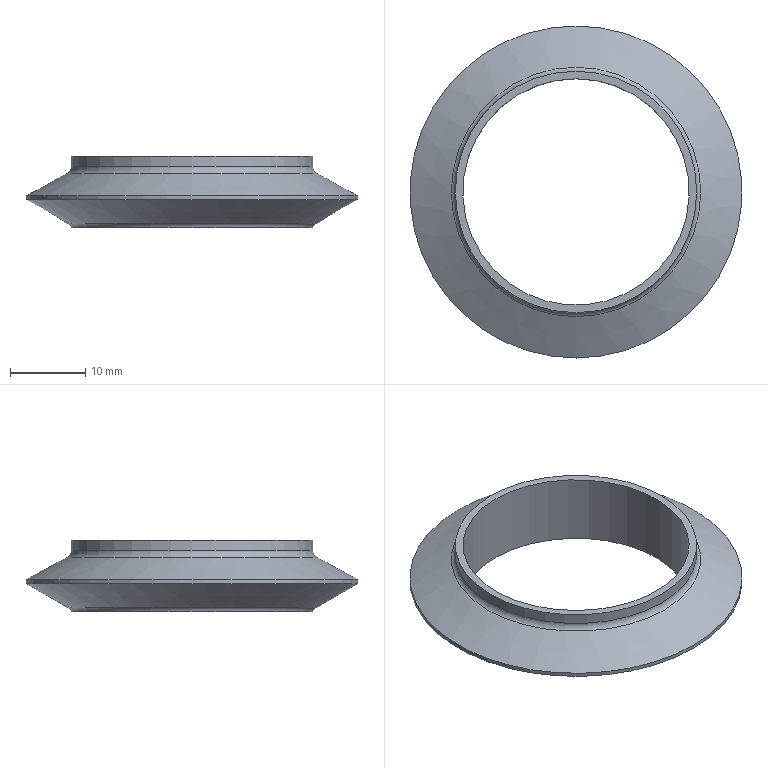Part | STEP file | 1-14.3 | 1 solid | 9 faces | box 44 x 44 x 9.5 mm | volume 3548 mm3 | cylinder 3 | cone 2 | torus 2 | plane 2 | commonest cylinder face diameters 30 x1 32 x1 44 x1
STEP:
#1=CARTESIAN_POINT('',(0.,0.,0.));
#2=DIRECTION('',(0.,0.,1.));
#3=DIRECTION('',(1.,0.,0.));
#4=AXIS2_PLACEMENT_3D('',#1,#2,#3);
#5=CARTESIAN_POINT('',(0.,22.,4.25));
#6=VERTEX_POINT('',#5);
#7=CARTESIAN_POINT('',(0.,0.,4.25));
#8=DIRECTION('',(0.,0.,1.));
#9=DIRECTION('',(0.,1.,0.));
#10=AXIS2_PLACEMENT_3D('',#7,#8,#9);
#11=CIRCLE('',#10,22.);
#12=CARTESIAN_POINT('',(0.,0.,7.216));
#13=DIRECTION('',(0.,0.,-1.));
#14=DIRECTION('',(0.,1.,0.));
#15=AXIS2_PLACEMENT_3D('',#12,#13,#14);
#16=CONICAL_SURFACE('',#15,16.524,1.074);
#17=CARTESIAN_POINT('',(6.283,2.966));
#18=DIRECTION('',(-1.,0.));
#19=VECTOR('',#18,1.);
#20=LINE('',#17,#19);
#21=(GEOMETRIC_REPRESENTATION_CONTEXT(2)PARAMETRIC_REPRESENTATION_CONTEXT()REPRESENTATION_CONTEXT('',''));
#22=DEFINITIONAL_REPRESENTATION('',(#20),#21);
#23=PCURVE('',#16,#22);
#24=CARTESIAN_POINT('',(0.,0.,3.75));
#25=DIRECTION('',(0.,0.,1.));
#26=DIRECTION('',(0.,1.,0.));
#27=AXIS2_PLACEMENT_3D('',#24,#25,#26);
#28=CYLINDRICAL_SURFACE('',#27,22.);
#29=CARTESIAN_POINT('',(0.,0.5));
#30=DIRECTION('',(1.,0.));
#31=VECTOR('',#30,1.);
#32=LINE('',#29,#31);
#33=(GEOMETRIC_REPRESENTATION_CONTEXT(2)PARAMETRIC_REPRESENTATION_CONTEXT()REPRESENTATION_CONTEXT('',''));
#34=DEFINITIONAL_REPRESENTATION('',(#32),#33);
#35=PCURVE('',#28,#34);
#36=SURFACE_CURVE('',#11,(#23,#35),.PCURVE_S1.);
#37=EDGE_CURVE('',#6,#6,#36,.T.);
#38=ORIENTED_EDGE('',*,*,#37,.T.);
#39=CARTESIAN_POINT('',(0.,16.524,7.216));
#40=VERTEX_POINT('',#39);
#41=CARTESIAN_POINT('',(0.,22.,4.25));
#42=DIRECTION('',(0.,-0.8793,0.4763));
#43=VECTOR('',#42,1.);
#44=LINE('',#41,#43);
#45=CARTESIAN_POINT('',(0.,2.966));
#46=DIRECTION('',(0.,-1.));
#47=VECTOR('',#46,1.);
#48=LINE('',#45,#47);
#49=(GEOMETRIC_REPRESENTATION_CONTEXT(2)PARAMETRIC_REPRESENTATION_CONTEXT()REPRESENTATION_CONTEXT('',''));
#50=DEFINITIONAL_REPRESENTATION('',(#48),#49);
#51=PCURVE('',#16,#50);
#52=CARTESIAN_POINT('',(6.283,2.966));
#53=DIRECTION('',(0.,-1.));
#54=VECTOR('',#53,1.);
#55=LINE('',#52,#54);
#56=(GEOMETRIC_REPRESENTATION_CONTEXT(2)PARAMETRIC_REPRESENTATION_CONTEXT()REPRESENTATION_CONTEXT('',''));
#57=DEFINITIONAL_REPRESENTATION('',(#55),#56);
#58=PCURVE('',#16,#57);
#59=SEAM_CURVE('',#44,(#51,#58),.PCURVE_S1.);
#60=EDGE_CURVE('',#6,#40,#59,.T.);
#61=ORIENTED_EDGE('',*,*,#60,.T.);
#62=CARTESIAN_POINT('',(0.,0.,7.216));
#63=DIRECTION('',(0.,0.,1.));
#64=DIRECTION('',(0.,1.,0.));
#65=AXIS2_PLACEMENT_3D('',#62,#63,#64);
#66=CIRCLE('',#65,16.524);
#67=CARTESIAN_POINT('',(6.283,0.));
#68=DIRECTION('',(-1.,0.));
#69=VECTOR('',#68,1.);
#70=LINE('',#67,#69);
#71=(GEOMETRIC_REPRESENTATION_CONTEXT(2)PARAMETRIC_REPRESENTATION_CONTEXT()REPRESENTATION_CONTEXT('',''));
#72=DEFINITIONAL_REPRESENTATION('',(#70),#71);
#73=PCURVE('',#16,#72);
#74=CARTESIAN_POINT('',(0.,0.,8.096));
#75=DIRECTION('',(0.,0.,-1.));
#76=DIRECTION('',(0.,1.,0.));
#77=AXIS2_PLACEMENT_3D('',#74,#75,#76);
#78=TOROIDAL_SURFACE('',#77,17.,1.);
#79=CARTESIAN_POINT('',(6.283,2.067));
#80=DIRECTION('',(-1.,0.));
#81=VECTOR('',#80,1.);
#82=LINE('',#79,#81);
#83=(GEOMETRIC_REPRESENTATION_CONTEXT(2)PARAMETRIC_REPRESENTATION_CONTEXT()REPRESENTATION_CONTEXT('',''));
#84=DEFINITIONAL_REPRESENTATION('',(#82),#83);
#85=PCURVE('',#78,#84);
#86=SURFACE_CURVE('',#66,(#73,#85),.PCURVE_S1.);
#87=EDGE_CURVE('',#40,#40,#86,.T.);
#88=ORIENTED_EDGE('',*,*,#87,.F.);
#89=ORIENTED_EDGE('',*,*,#60,.F.);
#90=EDGE_LOOP('',(#38,#61,#88,#89));
#91=FACE_BOUND('',#90,.T.);
#92=ADVANCED_FACE('',(#91),#16,.T.);
#93=CARTESIAN_POINT('',(0.,16.,8.096));
#94=VERTEX_POINT('',#93);
#95=CARTESIAN_POINT('',(0.,17.,8.096));
#96=DIRECTION('',(-1.,0.,0.));
#97=DIRECTION('',(0.,-0.4763,-0.8793));
#98=AXIS2_PLACEMENT_3D('',#95,#96,#97);
#99=CIRCLE('',#98,1.);
#100=CARTESIAN_POINT('',(6.283,2.067));
#101=DIRECTION('',(0.,1.));
#102=VECTOR('',#101,1.);
#103=LINE('',#100,#102);
#104=(GEOMETRIC_REPRESENTATION_CONTEXT(2)PARAMETRIC_REPRESENTATION_CONTEXT()REPRESENTATION_CONTEXT('',''));
#105=DEFINITIONAL_REPRESENTATION('',(#103),#104);
#106=PCURVE('',#78,#105);
#107=CARTESIAN_POINT('',(0.,2.067));
#108=DIRECTION('',(0.,1.));
#109=VECTOR('',#108,1.);
#110=LINE('',#107,#109);
#111=(GEOMETRIC_REPRESENTATION_CONTEXT(2)PARAMETRIC_REPRESENTATION_CONTEXT()REPRESENTATION_CONTEXT('',''));
#112=DEFINITIONAL_REPRESENTATION('',(#110),#111);
#113=PCURVE('',#78,#112);
#114=SEAM_CURVE('',#99,(#106,#113),.PCURVE_S1.);
#115=EDGE_CURVE('',#40,#94,#114,.T.);
#116=ORIENTED_EDGE('',*,*,#115,.T.);
#117=CARTESIAN_POINT('',(0.,0.,8.096));
#118=DIRECTION('',(0.,0.,1.));
#119=DIRECTION('',(0.,1.,0.));
#120=AXIS2_PLACEMENT_3D('',#117,#118,#119);
#121=CIRCLE('',#120,16.);
#122=CARTESIAN_POINT('',(6.283,3.142));
#123=DIRECTION('',(-1.,0.));
#124=VECTOR('',#123,1.);
#125=LINE('',#122,#124);
#126=(GEOMETRIC_REPRESENTATION_CONTEXT(2)PARAMETRIC_REPRESENTATION_CONTEXT()REPRESENTATION_CONTEXT('',''));
#127=DEFINITIONAL_REPRESENTATION('',(#125),#126);
#128=PCURVE('',#78,#127);
#129=CARTESIAN_POINT('',(0.,0.,8.096));
#130=DIRECTION('',(0.,0.,1.));
#131=DIRECTION('',(0.,1.,0.));
#132=AXIS2_PLACEMENT_3D('',#129,#130,#131);
#133=CYLINDRICAL_SURFACE('',#132,16.);
#134=CARTESIAN_POINT('',(0.,0.));
#135=DIRECTION('',(1.,0.));
#136=VECTOR('',#135,1.);
#137=LINE('',#134,#136);
#138=(GEOMETRIC_REPRESENTATION_CONTEXT(2)PARAMETRIC_REPRESENTATION_CONTEXT()REPRESENTATION_CONTEXT('',''));
#139=DEFINITIONAL_REPRESENTATION('',(#137),#138);
#140=PCURVE('',#133,#139);
#141=SURFACE_CURVE('',#121,(#128,#140),.PCURVE_S1.);
#142=EDGE_CURVE('',#94,#94,#141,.T.);
#143=ORIENTED_EDGE('',*,*,#142,.T.);
#144=ORIENTED_EDGE('',*,*,#115,.F.);
#145=ORIENTED_EDGE('',*,*,#87,.F.);
#146=EDGE_LOOP('',(#116,#143,#144,#145));
#147=FACE_BOUND('',#146,.F.);
#148=ADVANCED_FACE('',(#147),#78,.F.);
#149=ORIENTED_EDGE('',*,*,#142,.T.);
#150=CARTESIAN_POINT('',(0.,16.,9.5));
#151=VERTEX_POINT('',#150);
#152=CARTESIAN_POINT('',(0.,16.,8.096));
#153=DIRECTION('',(0.,0.,1.));
#154=VECTOR('',#153,1.);
#155=LINE('',#152,#154);
#156=CARTESIAN_POINT('',(6.283,0.));
#157=DIRECTION('',(0.,1.));
#158=VECTOR('',#157,1.);
#159=LINE('',#156,#158);
#160=(GEOMETRIC_REPRESENTATION_CONTEXT(2)PARAMETRIC_REPRESENTATION_CONTEXT()REPRESENTATION_CONTEXT('',''));
#161=DEFINITIONAL_REPRESENTATION('',(#159),#160);
#162=PCURVE('',#133,#161);
#163=CARTESIAN_POINT('',(0.,0.));
#164=DIRECTION('',(0.,1.));
#165=VECTOR('',#164,1.);
#166=LINE('',#163,#165);
#167=(GEOMETRIC_REPRESENTATION_CONTEXT(2)PARAMETRIC_REPRESENTATION_CONTEXT()REPRESENTATION_CONTEXT('',''));
#168=DEFINITIONAL_REPRESENTATION('',(#166),#167);
#169=PCURVE('',#133,#168);
#170=SEAM_CURVE('',#155,(#162,#169),.PCURVE_S1.);
#171=EDGE_CURVE('',#94,#151,#170,.T.);
#172=ORIENTED_EDGE('',*,*,#171,.T.);
#173=CARTESIAN_POINT('',(0.,0.,9.5));
#174=DIRECTION('',(0.,0.,1.));
#175=DIRECTION('',(0.,1.,0.));
#176=AXIS2_PLACEMENT_3D('',#173,#174,#175);
#177=CIRCLE('',#176,16.);
#178=CARTESIAN_POINT('',(0.,1.404));
#179=DIRECTION('',(1.,0.));
#180=VECTOR('',#179,1.);
#181=LINE('',#178,#180);
#182=(GEOMETRIC_REPRESENTATION_CONTEXT(2)PARAMETRIC_REPRESENTATION_CONTEXT()REPRESENTATION_CONTEXT('',''));
#183=DEFINITIONAL_REPRESENTATION('',(#181),#182);
#184=PCURVE('',#133,#183);
#185=CARTESIAN_POINT('',(0.,0.,9.5));
#186=DIRECTION('',(0.,0.,-1.));
#187=DIRECTION('',(0.,1.,0.));
#188=AXIS2_PLACEMENT_3D('',#185,#186,#187);
#189=PLANE('',#188);
#190=CARTESIAN_POINT('',(16.,0.));
#191=CARTESIAN_POINT('',(16.,-27.713));
#192=CARTESIAN_POINT('',(-8.,-13.856));
#193=CARTESIAN_POINT('',(-32.,0.));
#194=CARTESIAN_POINT('',(-8.,13.856));
#195=CARTESIAN_POINT('',(16.,27.713));
#196=CARTESIAN_POINT('',(16.,0.));
#197=(BOUNDED_CURVE()B_SPLINE_CURVE(2,(#190,#191,#192,#193,#194,#195,#196),.UNSPECIFIED.,.T.,.F.)B_SPLINE_CURVE_WITH_KNOTS((1,2,2,2,2,1),(-2.094,0.,2.094,4.189,6.283,8.378),.UNSPECIFIED.)CURVE()GEOMETRIC_REPRESENTATION_ITEM()RATIONAL_B_SPLINE_CURVE((1.,0.5,1.,0.5,1.,0.5,1.))REPRESENTATION_ITEM(''));
#198=(GEOMETRIC_REPRESENTATION_CONTEXT(2)PARAMETRIC_REPRESENTATION_CONTEXT()REPRESENTATION_CONTEXT('',''));
#199=DEFINITIONAL_REPRESENTATION('',(#197),#198);
#200=PCURVE('',#189,#199);
#201=SURFACE_CURVE('',#177,(#184,#200),.PCURVE_S1.);
#202=EDGE_CURVE('',#151,#151,#201,.T.);
#203=ORIENTED_EDGE('',*,*,#202,.F.);
#204=ORIENTED_EDGE('',*,*,#171,.F.);
#205=EDGE_LOOP('',(#149,#172,#203,#204));
#206=FACE_BOUND('',#205,.T.);
#207=ADVANCED_FACE('',(#206),#133,.T.);
#208=ORIENTED_EDGE('',*,*,#202,.F.);
#209=EDGE_LOOP('',(#208));
#210=FACE_BOUND('',#209,.F.);
#211=CARTESIAN_POINT('',(0.,15.,9.5));
#212=VERTEX_POINT('',#211);
#213=CARTESIAN_POINT('',(0.,0.,9.5));
#214=DIRECTION('',(0.,0.,1.));
#215=DIRECTION('',(0.,1.,0.));
#216=AXIS2_PLACEMENT_3D('',#213,#214,#215);
#217=CIRCLE('',#216,15.);
#218=CARTESIAN_POINT('',(15.,0.));
#219=CARTESIAN_POINT('',(15.,-25.981));
#220=CARTESIAN_POINT('',(-7.5,-12.99));
#221=CARTESIAN_POINT('',(-30.,0.));
#222=CARTESIAN_POINT('',(-7.5,12.99));
#223=CARTESIAN_POINT('',(15.,25.981));
#224=CARTESIAN_POINT('',(15.,0.));
#225=(BOUNDED_CURVE()B_SPLINE_CURVE(2,(#218,#219,#220,#221,#222,#223,#224),.UNSPECIFIED.,.T.,.F.)B_SPLINE_CURVE_WITH_KNOTS((1,2,2,2,2,1),(-2.094,0.,2.094,4.189,6.283,8.378),.UNSPECIFIED.)CURVE()GEOMETRIC_REPRESENTATION_ITEM()RATIONAL_B_SPLINE_CURVE((1.,0.5,1.,0.5,1.,0.5,1.))REPRESENTATION_ITEM(''));
#226=(GEOMETRIC_REPRESENTATION_CONTEXT(2)PARAMETRIC_REPRESENTATION_CONTEXT()REPRESENTATION_CONTEXT('',''));
#227=DEFINITIONAL_REPRESENTATION('',(#225),#226);
#228=PCURVE('',#189,#227);
#229=CARTESIAN_POINT('',(0.,0.,9.5));
#230=DIRECTION('',(0.,0.,-1.));
#231=DIRECTION('',(0.,1.,0.));
#232=AXIS2_PLACEMENT_3D('',#229,#230,#231);
#233=CYLINDRICAL_SURFACE('',#232,15.);
#234=CARTESIAN_POINT('',(6.283,0.));
#235=DIRECTION('',(-1.,0.));
#236=VECTOR('',#235,1.);
#237=LINE('',#234,#236);
#238=(GEOMETRIC_REPRESENTATION_CONTEXT(2)PARAMETRIC_REPRESENTATION_CONTEXT()REPRESENTATION_CONTEXT('',''));
#239=DEFINITIONAL_REPRESENTATION('',(#237),#238);
#240=PCURVE('',#233,#239);
#241=SURFACE_CURVE('',#217,(#228,#240),.PCURVE_S1.);
#242=EDGE_CURVE('',#212,#212,#241,.T.);
#243=ORIENTED_EDGE('',*,*,#242,.T.);
#244=EDGE_LOOP('',(#243));
#245=FACE_BOUND('',#244,.F.);
#246=ADVANCED_FACE('',(#210,#245),#189,.F.);
#247=CARTESIAN_POINT('',(0.,15.,0.));
#248=VERTEX_POINT('',#247);
#249=CARTESIAN_POINT('',(0.,15.,9.5));
#250=DIRECTION('',(0.,0.,-1.));
#251=VECTOR('',#250,1.);
#252=LINE('',#249,#251);
#253=CARTESIAN_POINT('',(6.283,0.));
#254=DIRECTION('',(0.,1.));
#255=VECTOR('',#254,1.);
#256=LINE('',#253,#255);
#257=(GEOMETRIC_REPRESENTATION_CONTEXT(2)PARAMETRIC_REPRESENTATION_CONTEXT()REPRESENTATION_CONTEXT('',''));
#258=DEFINITIONAL_REPRESENTATION('',(#256),#257);
#259=PCURVE('',#233,#258);
#260=CARTESIAN_POINT('',(0.,0.));
#261=DIRECTION('',(0.,1.));
#262=VECTOR('',#261,1.);
#263=LINE('',#260,#262);
#264=(GEOMETRIC_REPRESENTATION_CONTEXT(2)PARAMETRIC_REPRESENTATION_CONTEXT()REPRESENTATION_CONTEXT('',''));
#265=DEFINITIONAL_REPRESENTATION('',(#263),#264);
#266=PCURVE('',#233,#265);
#267=SEAM_CURVE('',#252,(#259,#266),.PCURVE_S1.);
#268=EDGE_CURVE('',#212,#248,#267,.T.);
#269=ORIENTED_EDGE('',*,*,#268,.T.);
#270=CARTESIAN_POINT('',(0.,0.,0.));
#271=DIRECTION('',(0.,0.,1.));
#272=DIRECTION('',(0.,1.,0.));
#273=AXIS2_PLACEMENT_3D('',#270,#271,#272);
#274=CIRCLE('',#273,15.);
#275=CARTESIAN_POINT('',(6.283,9.5));
#276=DIRECTION('',(-1.,0.));
#277=VECTOR('',#276,1.);
#278=LINE('',#275,#277);
#279=(GEOMETRIC_REPRESENTATION_CONTEXT(2)PARAMETRIC_REPRESENTATION_CONTEXT()REPRESENTATION_CONTEXT('',''));
#280=DEFINITIONAL_REPRESENTATION('',(#278),#279);
#281=PCURVE('',#233,#280);
#282=CARTESIAN_POINT('',(0.,0.,0.));
#283=DIRECTION('',(0.,0.,1.));
#284=DIRECTION('',(0.,1.,0.));
#285=AXIS2_PLACEMENT_3D('',#282,#283,#284);
#286=PLANE('',#285);
#287=CARTESIAN_POINT('',(0.,0.));
#288=DIRECTION('',(1.,0.));
#289=AXIS2_PLACEMENT_2D('',#287,#288);
#290=CIRCLE('',#289,15.);
#291=(GEOMETRIC_REPRESENTATION_CONTEXT(2)PARAMETRIC_REPRESENTATION_CONTEXT()REPRESENTATION_CONTEXT('',''));
#292=DEFINITIONAL_REPRESENTATION('',(#290),#291);
#293=PCURVE('',#286,#292);
#294=SURFACE_CURVE('',#274,(#281,#293),.PCURVE_S1.);
#295=EDGE_CURVE('',#248,#248,#294,.T.);
#296=ORIENTED_EDGE('',*,*,#295,.T.);
#297=ORIENTED_EDGE('',*,*,#268,.F.);
#298=ORIENTED_EDGE('',*,*,#242,.F.);
#299=EDGE_LOOP('',(#269,#296,#297,#298));
#300=FACE_BOUND('',#299,.F.);
#301=ADVANCED_FACE('',(#300),#233,.F.);
#302=CARTESIAN_POINT('',(0.,16.,0.));
#303=VERTEX_POINT('',#302);
#304=CARTESIAN_POINT('',(0.,0.,0.));
#305=DIRECTION('',(0.,0.,1.));
#306=DIRECTION('',(0.,1.,0.));
#307=AXIS2_PLACEMENT_3D('',#304,#305,#306);
#308=CIRCLE('',#307,16.);
#309=CARTESIAN_POINT('',(0.,0.));
#310=DIRECTION('',(1.,0.));
#311=AXIS2_PLACEMENT_2D('',#309,#310);
#312=CIRCLE('',#311,16.);
#313=(GEOMETRIC_REPRESENTATION_CONTEXT(2)PARAMETRIC_REPRESENTATION_CONTEXT()REPRESENTATION_CONTEXT('',''));
#314=DEFINITIONAL_REPRESENTATION('',(#312),#313);
#315=PCURVE('',#286,#314);
#316=CARTESIAN_POINT('',(0.,0.,0.));
#317=DIRECTION('',(0.,0.,-1.));
#318=DIRECTION('',(0.,1.,0.));
#319=AXIS2_PLACEMENT_3D('',#316,#317,#318);
#320=TOROIDAL_SURFACE('',#319,16.6,0.6);
#321=CARTESIAN_POINT('',(6.283,3.142));
#322=DIRECTION('',(-1.,0.));
#323=VECTOR('',#322,1.);
#324=LINE('',#321,#323);
#325=(GEOMETRIC_REPRESENTATION_CONTEXT(2)PARAMETRIC_REPRESENTATION_CONTEXT()REPRESENTATION_CONTEXT('',''));
#326=DEFINITIONAL_REPRESENTATION('',(#324),#325);
#327=PCURVE('',#320,#326);
#328=SURFACE_CURVE('',#308,(#315,#327),.PCURVE_S1.);
#329=EDGE_CURVE('',#303,#303,#328,.T.);
#330=ORIENTED_EDGE('',*,*,#329,.T.);
#331=EDGE_LOOP('',(#330));
#332=FACE_BOUND('',#331,.F.);
#333=ORIENTED_EDGE('',*,*,#295,.F.);
#334=EDGE_LOOP('',(#333));
#335=FACE_BOUND('',#334,.F.);
#336=ADVANCED_FACE('',(#332,#335),#286,.F.);
#337=CARTESIAN_POINT('',(0.,16.304,0.522));
#338=VERTEX_POINT('',#337);
#339=CARTESIAN_POINT('',(0.,16.6,0.));
#340=DIRECTION('',(-1.,0.,0.));
#341=DIRECTION('',(0.,-1.,0.));
#342=AXIS2_PLACEMENT_3D('',#339,#340,#341);
#343=CIRCLE('',#342,0.6);
#344=CARTESIAN_POINT('',(6.283,3.142));
#345=DIRECTION('',(0.,1.));
#346=VECTOR('',#345,1.);
#347=LINE('',#344,#346);
#348=(GEOMETRIC_REPRESENTATION_CONTEXT(2)PARAMETRIC_REPRESENTATION_CONTEXT()REPRESENTATION_CONTEXT('',''));
#349=DEFINITIONAL_REPRESENTATION('',(#347),#348);
#350=PCURVE('',#320,#349);
#351=CARTESIAN_POINT('',(0.,3.142));
#352=DIRECTION('',(0.,1.));
#353=VECTOR('',#352,1.);
#354=LINE('',#351,#353);
#355=(GEOMETRIC_REPRESENTATION_CONTEXT(2)PARAMETRIC_REPRESENTATION_CONTEXT()REPRESENTATION_CONTEXT('',''));
#356=DEFINITIONAL_REPRESENTATION('',(#354),#355);
#357=PCURVE('',#320,#356);
#358=SEAM_CURVE('',#343,(#350,#357),.PCURVE_S1.);
#359=EDGE_CURVE('',#303,#338,#358,.T.);
#360=ORIENTED_EDGE('',*,*,#359,.T.);
#361=CARTESIAN_POINT('',(0.,0.,0.522));
#362=DIRECTION('',(0.,0.,1.));
#363=DIRECTION('',(0.,1.,0.));
#364=AXIS2_PLACEMENT_3D('',#361,#362,#363);
#365=CIRCLE('',#364,16.304);
#366=CARTESIAN_POINT('',(6.283,4.197));
#367=DIRECTION('',(-1.,0.));
#368=VECTOR('',#367,1.);
#369=LINE('',#366,#368);
#370=(GEOMETRIC_REPRESENTATION_CONTEXT(2)PARAMETRIC_REPRESENTATION_CONTEXT()REPRESENTATION_CONTEXT('',''));
#371=DEFINITIONAL_REPRESENTATION('',(#369),#370);
#372=PCURVE('',#320,#371);
#373=CARTESIAN_POINT('',(0.,0.,0.522));
#374=DIRECTION('',(0.,0.,1.));
#375=DIRECTION('',(0.,1.,0.));
#376=AXIS2_PLACEMENT_3D('',#373,#374,#375);
#377=CONICAL_SURFACE('',#376,16.304,1.055);
#378=CARTESIAN_POINT('',(0.,0.));
#379=DIRECTION('',(1.,0.));
#380=VECTOR('',#379,1.);
#381=LINE('',#378,#380);
#382=(GEOMETRIC_REPRESENTATION_CONTEXT(2)PARAMETRIC_REPRESENTATION_CONTEXT()REPRESENTATION_CONTEXT('',''));
#383=DEFINITIONAL_REPRESENTATION('',(#381),#382);
#384=PCURVE('',#377,#383);
#385=SURFACE_CURVE('',#365,(#372,#384),.PCURVE_S1.);
#386=EDGE_CURVE('',#338,#338,#385,.T.);
#387=ORIENTED_EDGE('',*,*,#386,.T.);
#388=ORIENTED_EDGE('',*,*,#359,.F.);
#389=ORIENTED_EDGE('',*,*,#329,.F.);
#390=EDGE_LOOP('',(#360,#387,#388,#389));
#391=FACE_BOUND('',#390,.F.);
#392=ADVANCED_FACE('',(#391),#320,.F.);
#393=ORIENTED_EDGE('',*,*,#386,.T.);
#394=CARTESIAN_POINT('',(0.,22.,3.75));
#395=VERTEX_POINT('',#394);
#396=CARTESIAN_POINT('',(0.,16.304,0.522));
#397=DIRECTION('',(0.,0.87,0.4931));
#398=VECTOR('',#397,1.);
#399=LINE('',#396,#398);
#400=CARTESIAN_POINT('',(6.283,0.));
#401=DIRECTION('',(0.,1.));
#402=VECTOR('',#401,1.);
#403=LINE('',#400,#402);
#404=(GEOMETRIC_REPRESENTATION_CONTEXT(2)PARAMETRIC_REPRESENTATION_CONTEXT()REPRESENTATION_CONTEXT('',''));
#405=DEFINITIONAL_REPRESENTATION('',(#403),#404);
#406=PCURVE('',#377,#405);
#407=CARTESIAN_POINT('',(0.,0.));
#408=DIRECTION('',(0.,1.));
#409=VECTOR('',#408,1.);
#410=LINE('',#407,#409);
#411=(GEOMETRIC_REPRESENTATION_CONTEXT(2)PARAMETRIC_REPRESENTATION_CONTEXT()REPRESENTATION_CONTEXT('',''));
#412=DEFINITIONAL_REPRESENTATION('',(#410),#411);
#413=PCURVE('',#377,#412);
#414=SEAM_CURVE('',#399,(#406,#413),.PCURVE_S1.);
#415=EDGE_CURVE('',#338,#395,#414,.T.);
#416=ORIENTED_EDGE('',*,*,#415,.T.);
#417=CARTESIAN_POINT('',(0.,0.,3.75));
#418=DIRECTION('',(0.,0.,1.));
#419=DIRECTION('',(0.,1.,0.));
#420=AXIS2_PLACEMENT_3D('',#417,#418,#419);
#421=CIRCLE('',#420,22.);
#422=CARTESIAN_POINT('',(0.,3.228));
#423=DIRECTION('',(1.,0.));
#424=VECTOR('',#423,1.);
#425=LINE('',#422,#424);
#426=(GEOMETRIC_REPRESENTATION_CONTEXT(2)PARAMETRIC_REPRESENTATION_CONTEXT()REPRESENTATION_CONTEXT('',''));
#427=DEFINITIONAL_REPRESENTATION('',(#425),#426);
#428=PCURVE('',#377,#427);
#429=CARTESIAN_POINT('',(0.,0.));
#430=DIRECTION('',(1.,0.));
#431=VECTOR('',#430,1.);
#432=LINE('',#429,#431);
#433=(GEOMETRIC_REPRESENTATION_CONTEXT(2)PARAMETRIC_REPRESENTATION_CONTEXT()REPRESENTATION_CONTEXT('',''));
#434=DEFINITIONAL_REPRESENTATION('',(#432),#433);
#435=PCURVE('',#28,#434);
#436=SURFACE_CURVE('',#421,(#428,#435),.PCURVE_S1.);
#437=EDGE_CURVE('',#395,#395,#436,.T.);
#438=ORIENTED_EDGE('',*,*,#437,.F.);
#439=ORIENTED_EDGE('',*,*,#415,.F.);
#440=EDGE_LOOP('',(#393,#416,#438,#439));
#441=FACE_BOUND('',#440,.T.);
#442=ADVANCED_FACE('',(#441),#377,.T.);
#443=ORIENTED_EDGE('',*,*,#437,.T.);
#444=CARTESIAN_POINT('',(0.,22.,3.75));
#445=DIRECTION('',(0.,0.,1.));
#446=VECTOR('',#445,1.);
#447=LINE('',#444,#446);
#448=CARTESIAN_POINT('',(6.283,0.));
#449=DIRECTION('',(0.,1.));
#450=VECTOR('',#449,1.);
#451=LINE('',#448,#450);
#452=(GEOMETRIC_REPRESENTATION_CONTEXT(2)PARAMETRIC_REPRESENTATION_CONTEXT()REPRESENTATION_CONTEXT('',''));
#453=DEFINITIONAL_REPRESENTATION('',(#451),#452);
#454=PCURVE('',#28,#453);
#455=CARTESIAN_POINT('',(0.,0.));
#456=DIRECTION('',(0.,1.));
#457=VECTOR('',#456,1.);
#458=LINE('',#455,#457);
#459=(GEOMETRIC_REPRESENTATION_CONTEXT(2)PARAMETRIC_REPRESENTATION_CONTEXT()REPRESENTATION_CONTEXT('',''));
#460=DEFINITIONAL_REPRESENTATION('',(#458),#459);
#461=PCURVE('',#28,#460);
#462=SEAM_CURVE('',#447,(#454,#461),.PCURVE_S1.);
#463=EDGE_CURVE('',#395,#6,#462,.T.);
#464=ORIENTED_EDGE('',*,*,#463,.T.);
#465=ORIENTED_EDGE('',*,*,#37,.F.);
#466=ORIENTED_EDGE('',*,*,#463,.F.);
#467=EDGE_LOOP('',(#443,#464,#465,#466));
#468=FACE_BOUND('',#467,.T.);
#469=ADVANCED_FACE('',(#468),#28,.T.);
#470=CLOSED_SHELL('',(#92,#148,#207,#246,#301,#336,#392,#442,#469));
#471=MANIFOLD_SOLID_BREP('',#470);
#472=(LENGTH_UNIT()NAMED_UNIT(*)SI_UNIT(.MILLI.,.METRE.));
#473=UNCERTAINTY_MEASURE_WITH_UNIT(LENGTH_MEASURE(0.0000001),#472,'','');
#474=(NAMED_UNIT(*)PLANE_ANGLE_UNIT()SI_UNIT($,.RADIAN.));
#475=(NAMED_UNIT(*)SI_UNIT($,.STERADIAN.)SOLID_ANGLE_UNIT());
#476=(GEOMETRIC_REPRESENTATION_CONTEXT(3)GLOBAL_UNCERTAINTY_ASSIGNED_CONTEXT((#473))GLOBAL_UNIT_ASSIGNED_CONTEXT((#472,#474,#475))REPRESENTATION_CONTEXT('',''));
#477=ADVANCED_BREP_SHAPE_REPRESENTATION('',(#4,#471),#476);